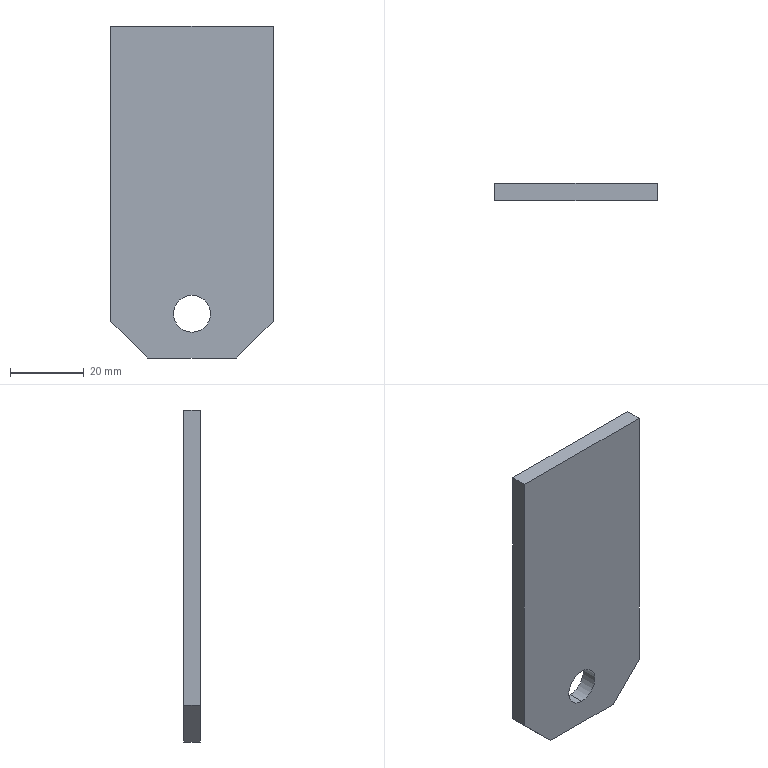Part | SolidWorks | features FlatPattern 1, SMBaseFlange 1, SheetMetal 1 | 1 solid | 10 faces | box 44 x 4.5 x 90 mm | volume 17017 mm3 | plane 8 | cylinder 2 | commonest cylinder face diameters 10 x2
STEP:
#1=CARTESIAN_POINT('',(0.,-4.5,-38.));
#2=VERTEX_POINT('',#1);
#3=CARTESIAN_POINT('',(0.,-4.5,-28.));
#4=VERTEX_POINT('',#3);
#5=CARTESIAN_POINT('',(0.,-4.5,-33.));
#6=DIRECTION('',(0.,1.,0.));
#7=DIRECTION('',(0.,0.,1.));
#8=AXIS2_PLACEMENT_3D('',#5,#6,#7);
#9=CIRCLE('',#8,5.);
#10=EDGE_CURVE('',#2,#4,#9,.T.);
#11=ORIENTED_EDGE('',*,*,#10,.F.);
#12=CARTESIAN_POINT('',(0.,0.,-38.));
#13=VERTEX_POINT('',#12);
#14=CARTESIAN_POINT('',(0.,-4.5,-38.));
#15=DIRECTION('',(0.,1.,0.));
#16=VECTOR('',#15,1000.);
#17=LINE('',#14,#16);
#18=EDGE_CURVE('',#2,#13,#17,.T.);
#19=ORIENTED_EDGE('',*,*,#18,.T.);
#20=CARTESIAN_POINT('',(0.,0.,-28.));
#21=VERTEX_POINT('',#20);
#22=CARTESIAN_POINT('',(0.,0.,-33.));
#23=DIRECTION('',(0.,1.,0.));
#24=DIRECTION('',(0.,0.,1.));
#25=AXIS2_PLACEMENT_3D('',#22,#23,#24);
#26=CIRCLE('',#25,5.);
#27=EDGE_CURVE('',#13,#21,#26,.T.);
#28=ORIENTED_EDGE('',*,*,#27,.T.);
#29=CARTESIAN_POINT('',(0.,-4.5,-28.));
#30=DIRECTION('',(0.,1.,0.));
#31=VECTOR('',#30,1000.);
#32=LINE('',#29,#31);
#33=EDGE_CURVE('',#4,#21,#32,.T.);
#34=ORIENTED_EDGE('',*,*,#33,.F.);
#35=EDGE_LOOP('',(#11,#19,#28,#34));
#36=FACE_OUTER_BOUND('',#35,.T.);
#37=CARTESIAN_POINT('',(0.,-4.5,-33.));
#38=DIRECTION('',(0.,1.,0.));
#39=DIRECTION('',(0.,0.,1.));
#40=AXIS2_PLACEMENT_3D('',#37,#38,#39);
#41=CYLINDRICAL_SURFACE('',#40,5.);
#42=ADVANCED_FACE('',(#36),#41,.F.);
#43=CARTESIAN_POINT('',(22.,0.,45.));
#44=VERTEX_POINT('',#43);
#45=CARTESIAN_POINT('',(22.,0.,-35.));
#46=VERTEX_POINT('',#45);
#47=CARTESIAN_POINT('',(22.,0.,-35.));
#48=DIRECTION('',(0.,0.,-1.));
#49=VECTOR('',#48,1000.);
#50=LINE('',#47,#49);
#51=EDGE_CURVE('',#44,#46,#50,.T.);
#52=ORIENTED_EDGE('',*,*,#51,.F.);
#53=CARTESIAN_POINT('',(22.,-4.5,45.));
#54=VERTEX_POINT('',#53);
#55=CARTESIAN_POINT('',(22.,-4.5,45.));
#56=DIRECTION('',(0.,1.,0.));
#57=VECTOR('',#56,1000.);
#58=LINE('',#55,#57);
#59=EDGE_CURVE('',#54,#44,#58,.T.);
#60=ORIENTED_EDGE('',*,*,#59,.F.);
#61=CARTESIAN_POINT('',(22.,-4.5,-35.));
#62=VERTEX_POINT('',#61);
#63=CARTESIAN_POINT('',(22.,-4.5,-35.));
#64=DIRECTION('',(0.,0.,-1.));
#65=VECTOR('',#64,1000.);
#66=LINE('',#63,#65);
#67=EDGE_CURVE('',#54,#62,#66,.T.);
#68=ORIENTED_EDGE('',*,*,#67,.T.);
#69=CARTESIAN_POINT('',(22.,-4.5,-35.));
#70=DIRECTION('',(0.,1.,0.));
#71=VECTOR('',#70,1000.);
#72=LINE('',#69,#71);
#73=EDGE_CURVE('',#62,#46,#72,.T.);
#74=ORIENTED_EDGE('',*,*,#73,.T.);
#75=EDGE_LOOP('',(#52,#60,#68,#74));
#76=FACE_OUTER_BOUND('',#75,.T.);
#77=CARTESIAN_POINT('',(22.,-4.5,-35.));
#78=DIRECTION('',(1.,0.,0.));
#79=DIRECTION('',(0.,0.,-1.));
#80=AXIS2_PLACEMENT_3D('',#77,#78,#79);
#81=PLANE('',#80);
#82=ADVANCED_FACE('',(#76),#81,.T.);
#83=CARTESIAN_POINT('',(-22.,0.,45.));
#84=VERTEX_POINT('',#83);
#85=CARTESIAN_POINT('',(-22.,0.,45.));
#86=DIRECTION('',(1.,0.,0.));
#87=VECTOR('',#86,1000.);
#88=LINE('',#85,#87);
#89=EDGE_CURVE('',#84,#44,#88,.T.);
#90=ORIENTED_EDGE('',*,*,#89,.F.);
#91=CARTESIAN_POINT('',(-22.,-4.5,45.));
#92=VERTEX_POINT('',#91);
#93=CARTESIAN_POINT('',(-22.,-4.5,45.));
#94=DIRECTION('',(0.,1.,0.));
#95=VECTOR('',#94,1000.);
#96=LINE('',#93,#95);
#97=EDGE_CURVE('',#92,#84,#96,.T.);
#98=ORIENTED_EDGE('',*,*,#97,.F.);
#99=CARTESIAN_POINT('',(-22.,-4.5,45.));
#100=DIRECTION('',(1.,0.,0.));
#101=VECTOR('',#100,1000.);
#102=LINE('',#99,#101);
#103=EDGE_CURVE('',#92,#54,#102,.T.);
#104=ORIENTED_EDGE('',*,*,#103,.T.);
#105=ORIENTED_EDGE('',*,*,#59,.T.);
#106=EDGE_LOOP('',(#90,#98,#104,#105));
#107=FACE_OUTER_BOUND('',#106,.T.);
#108=CARTESIAN_POINT('',(-22.,-4.5,45.));
#109=DIRECTION('',(0.,0.,1.));
#110=DIRECTION('',(1.,0.,0.));
#111=AXIS2_PLACEMENT_3D('',#108,#109,#110);
#112=PLANE('',#111);
#113=ADVANCED_FACE('',(#107),#112,.T.);
#114=CARTESIAN_POINT('',(-22.,0.,-35.));
#115=VERTEX_POINT('',#114);
#116=CARTESIAN_POINT('',(-22.,0.,-35.));
#117=DIRECTION('',(0.,0.,1.));
#118=VECTOR('',#117,1000.);
#119=LINE('',#116,#118);
#120=EDGE_CURVE('',#115,#84,#119,.T.);
#121=ORIENTED_EDGE('',*,*,#120,.F.);
#122=CARTESIAN_POINT('',(-22.,-4.5,-35.));
#123=VERTEX_POINT('',#122);
#124=CARTESIAN_POINT('',(-22.,-4.5,-35.));
#125=DIRECTION('',(0.,1.,0.));
#126=VECTOR('',#125,1000.);
#127=LINE('',#124,#126);
#128=EDGE_CURVE('',#123,#115,#127,.T.);
#129=ORIENTED_EDGE('',*,*,#128,.F.);
#130=CARTESIAN_POINT('',(-22.,-4.5,-35.));
#131=DIRECTION('',(0.,0.,1.));
#132=VECTOR('',#131,1000.);
#133=LINE('',#130,#132);
#134=EDGE_CURVE('',#123,#92,#133,.T.);
#135=ORIENTED_EDGE('',*,*,#134,.T.);
#136=ORIENTED_EDGE('',*,*,#97,.T.);
#137=EDGE_LOOP('',(#121,#129,#135,#136));
#138=FACE_OUTER_BOUND('',#137,.T.);
#139=CARTESIAN_POINT('',(-22.,-4.5,-35.));
#140=DIRECTION('',(-1.,0.,0.));
#141=DIRECTION('',(0.,0.,1.));
#142=AXIS2_PLACEMENT_3D('',#139,#140,#141);
#143=PLANE('',#142);
#144=ADVANCED_FACE('',(#138),#143,.T.);
#145=CARTESIAN_POINT('',(-12.,0.,-45.));
#146=VERTEX_POINT('',#145);
#147=CARTESIAN_POINT('',(-22.,0.,-35.));
#148=DIRECTION('',(-0.7071,0.,0.7071));
#149=VECTOR('',#148,1000.);
#150=LINE('',#147,#149);
#151=EDGE_CURVE('',#146,#115,#150,.T.);
#152=ORIENTED_EDGE('',*,*,#151,.F.);
#153=CARTESIAN_POINT('',(-12.,-4.5,-45.));
#154=VERTEX_POINT('',#153);
#155=CARTESIAN_POINT('',(-12.,-4.5,-45.));
#156=DIRECTION('',(0.,1.,0.));
#157=VECTOR('',#156,1000.);
#158=LINE('',#155,#157);
#159=EDGE_CURVE('',#154,#146,#158,.T.);
#160=ORIENTED_EDGE('',*,*,#159,.F.);
#161=CARTESIAN_POINT('',(-22.,-4.5,-35.));
#162=DIRECTION('',(-0.7071,0.,0.7071));
#163=VECTOR('',#162,1000.);
#164=LINE('',#161,#163);
#165=EDGE_CURVE('',#154,#123,#164,.T.);
#166=ORIENTED_EDGE('',*,*,#165,.T.);
#167=ORIENTED_EDGE('',*,*,#128,.T.);
#168=EDGE_LOOP('',(#152,#160,#166,#167));
#169=FACE_OUTER_BOUND('',#168,.T.);
#170=CARTESIAN_POINT('',(-22.,-4.5,-35.));
#171=DIRECTION('',(-0.7071,0.,-0.7071));
#172=DIRECTION('',(-0.7071,0.,0.7071));
#173=AXIS2_PLACEMENT_3D('',#170,#171,#172);
#174=PLANE('',#173);
#175=ADVANCED_FACE('',(#169),#174,.T.);
#176=CARTESIAN_POINT('',(12.,0.,-45.));
#177=VERTEX_POINT('',#176);
#178=CARTESIAN_POINT('',(-12.,0.,-45.));
#179=DIRECTION('',(-1.,0.,0.));
#180=VECTOR('',#179,1000.);
#181=LINE('',#178,#180);
#182=EDGE_CURVE('',#177,#146,#181,.T.);
#183=ORIENTED_EDGE('',*,*,#182,.F.);
#184=CARTESIAN_POINT('',(12.,-4.5,-45.));
#185=VERTEX_POINT('',#184);
#186=CARTESIAN_POINT('',(12.,-4.5,-45.));
#187=DIRECTION('',(0.,1.,0.));
#188=VECTOR('',#187,1000.);
#189=LINE('',#186,#188);
#190=EDGE_CURVE('',#185,#177,#189,.T.);
#191=ORIENTED_EDGE('',*,*,#190,.F.);
#192=CARTESIAN_POINT('',(-12.,-4.5,-45.));
#193=DIRECTION('',(-1.,0.,0.));
#194=VECTOR('',#193,1000.);
#195=LINE('',#192,#194);
#196=EDGE_CURVE('',#185,#154,#195,.T.);
#197=ORIENTED_EDGE('',*,*,#196,.T.);
#198=ORIENTED_EDGE('',*,*,#159,.T.);
#199=EDGE_LOOP('',(#183,#191,#197,#198));
#200=FACE_OUTER_BOUND('',#199,.T.);
#201=CARTESIAN_POINT('',(-12.,-4.5,-45.));
#202=DIRECTION('',(0.,0.,-1.));
#203=DIRECTION('',(-1.,0.,0.));
#204=AXIS2_PLACEMENT_3D('',#201,#202,#203);
#205=PLANE('',#204);
#206=ADVANCED_FACE('',(#200),#205,.T.);
#207=CARTESIAN_POINT('',(12.,0.,-45.));
#208=DIRECTION('',(-0.7071,0.,-0.7071));
#209=VECTOR('',#208,1000.);
#210=LINE('',#207,#209);
#211=EDGE_CURVE('',#46,#177,#210,.T.);
#212=ORIENTED_EDGE('',*,*,#211,.F.);
#213=ORIENTED_EDGE('',*,*,#73,.F.);
#214=CARTESIAN_POINT('',(12.,-4.5,-45.));
#215=DIRECTION('',(-0.7071,0.,-0.7071));
#216=VECTOR('',#215,1000.);
#217=LINE('',#214,#216);
#218=EDGE_CURVE('',#62,#185,#217,.T.);
#219=ORIENTED_EDGE('',*,*,#218,.T.);
#220=ORIENTED_EDGE('',*,*,#190,.T.);
#221=EDGE_LOOP('',(#212,#213,#219,#220));
#222=FACE_OUTER_BOUND('',#221,.T.);
#223=CARTESIAN_POINT('',(12.,-4.5,-45.));
#224=DIRECTION('',(0.7071,0.,-0.7071));
#225=DIRECTION('',(-0.7071,0.,-0.7071));
#226=AXIS2_PLACEMENT_3D('',#223,#224,#225);
#227=PLANE('',#226);
#228=ADVANCED_FACE('',(#222),#227,.T.);
#229=CARTESIAN_POINT('',(0.,-4.5,-33.));
#230=DIRECTION('',(0.,1.,0.));
#231=DIRECTION('',(0.,0.,1.));
#232=AXIS2_PLACEMENT_3D('',#229,#230,#231);
#233=CIRCLE('',#232,5.);
#234=EDGE_CURVE('',#4,#2,#233,.T.);
#235=ORIENTED_EDGE('',*,*,#234,.T.);
#236=ORIENTED_EDGE('',*,*,#10,.T.);
#237=EDGE_LOOP('',(#235,#236));
#238=FACE_BOUND('',#237,.T.);
#239=ORIENTED_EDGE('',*,*,#67,.F.);
#240=ORIENTED_EDGE('',*,*,#103,.F.);
#241=ORIENTED_EDGE('',*,*,#134,.F.);
#242=ORIENTED_EDGE('',*,*,#165,.F.);
#243=ORIENTED_EDGE('',*,*,#196,.F.);
#244=ORIENTED_EDGE('',*,*,#218,.F.);
#245=EDGE_LOOP('',(#239,#240,#241,#242,#243,#244));
#246=FACE_OUTER_BOUND('',#245,.T.);
#247=CARTESIAN_POINT('',(0.,-4.5,0.));
#248=DIRECTION('',(0.,1.,0.));
#249=DIRECTION('',(0.,0.,1.));
#250=AXIS2_PLACEMENT_3D('',#247,#248,#249);
#251=PLANE('',#250);
#252=ADVANCED_FACE('',(#238,#246),#251,.F.);
#253=CARTESIAN_POINT('',(0.,0.,-33.));
#254=DIRECTION('',(0.,1.,0.));
#255=DIRECTION('',(0.,0.,1.));
#256=AXIS2_PLACEMENT_3D('',#253,#254,#255);
#257=CIRCLE('',#256,5.);
#258=EDGE_CURVE('',#21,#13,#257,.T.);
#259=ORIENTED_EDGE('',*,*,#258,.F.);
#260=ORIENTED_EDGE('',*,*,#27,.F.);
#261=EDGE_LOOP('',(#259,#260));
#262=FACE_BOUND('',#261,.T.);
#263=ORIENTED_EDGE('',*,*,#51,.T.);
#264=ORIENTED_EDGE('',*,*,#211,.T.);
#265=ORIENTED_EDGE('',*,*,#182,.T.);
#266=ORIENTED_EDGE('',*,*,#151,.T.);
#267=ORIENTED_EDGE('',*,*,#120,.T.);
#268=ORIENTED_EDGE('',*,*,#89,.T.);
#269=EDGE_LOOP('',(#263,#264,#265,#266,#267,#268));
#270=FACE_OUTER_BOUND('',#269,.T.);
#271=CARTESIAN_POINT('',(0.,0.,0.));
#272=DIRECTION('',(0.,1.,0.));
#273=DIRECTION('',(0.,0.,1.));
#274=AXIS2_PLACEMENT_3D('',#271,#272,#273);
#275=PLANE('',#274);
#276=ADVANCED_FACE('',(#262,#270),#275,.T.);
#277=ORIENTED_EDGE('',*,*,#18,.F.);
#278=ORIENTED_EDGE('',*,*,#234,.F.);
#279=ORIENTED_EDGE('',*,*,#33,.T.);
#280=ORIENTED_EDGE('',*,*,#258,.T.);
#281=EDGE_LOOP('',(#277,#278,#279,#280));
#282=FACE_OUTER_BOUND('',#281,.T.);
#283=CARTESIAN_POINT('',(0.,-4.5,-33.));
#284=DIRECTION('',(0.,1.,0.));
#285=DIRECTION('',(0.,0.,1.));
#286=AXIS2_PLACEMENT_3D('',#283,#284,#285);
#287=CYLINDRICAL_SURFACE('',#286,5.);
#288=ADVANCED_FACE('',(#282),#287,.F.);
#289=CLOSED_SHELL('',(#42,#82,#113,#144,#175,#206,#228,#252,#276,#288));
#290=MANIFOLD_SOLID_BREP('',#289);
#291=CARTESIAN_POINT('',(0.,0.,0.));
#292=DIRECTION('',(0.,0.,1.));
#293=DIRECTION('',(1.,0.,0.));
#294=AXIS2_PLACEMENT_3D('',#291,#292,#293);
#295=(LENGTH_UNIT()NAMED_UNIT(*)SI_UNIT(.MILLI.,.METRE.));
#296=UNCERTAINTY_MEASURE_WITH_UNIT(LENGTH_MEASURE(0.00001),#295,'','');
#297=(NAMED_UNIT(*)PLANE_ANGLE_UNIT()SI_UNIT($,.RADIAN.));
#298=(NAMED_UNIT(*)SI_UNIT($,.STERADIAN.)SOLID_ANGLE_UNIT());
#299=(GEOMETRIC_REPRESENTATION_CONTEXT(3)GLOBAL_UNCERTAINTY_ASSIGNED_CONTEXT((#296))GLOBAL_UNIT_ASSIGNED_CONTEXT((#295,#297,#298))REPRESENTATION_CONTEXT('',''));
#300=ADVANCED_BREP_SHAPE_REPRESENTATION('',(#290,#294),#299);